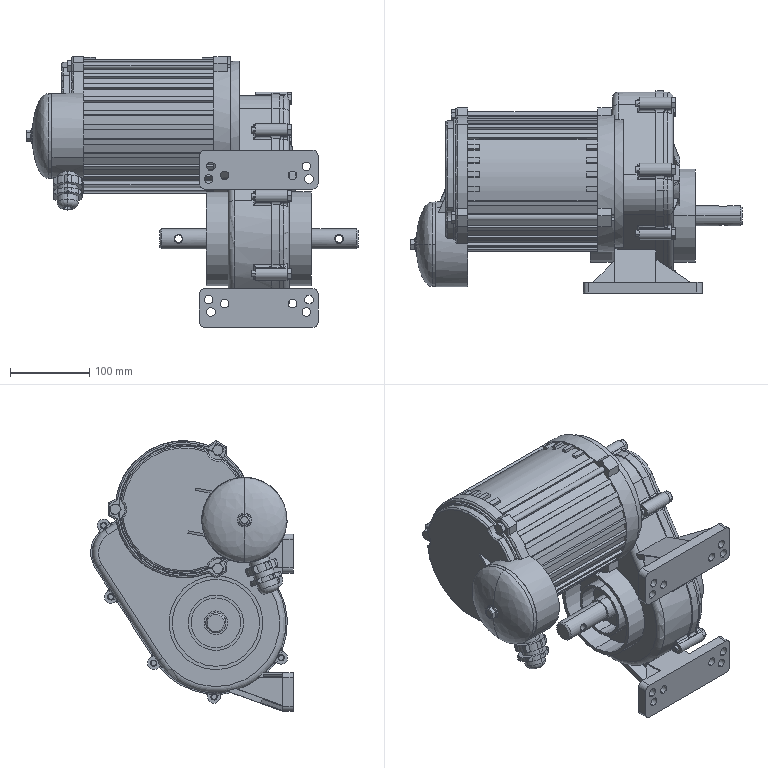Part | SolidWorks | 16 solids | 1120 faces | box 419.954 x 256.191 x 342.427 mm | volume 6353002 mm3 | plane 552 | cylinder 324 | cone 139 | torus 66 | spline 39 | commonest cylinder face diameters 6 x113 8 x36 11 x24 2 x16 16 x12 37.4 x12